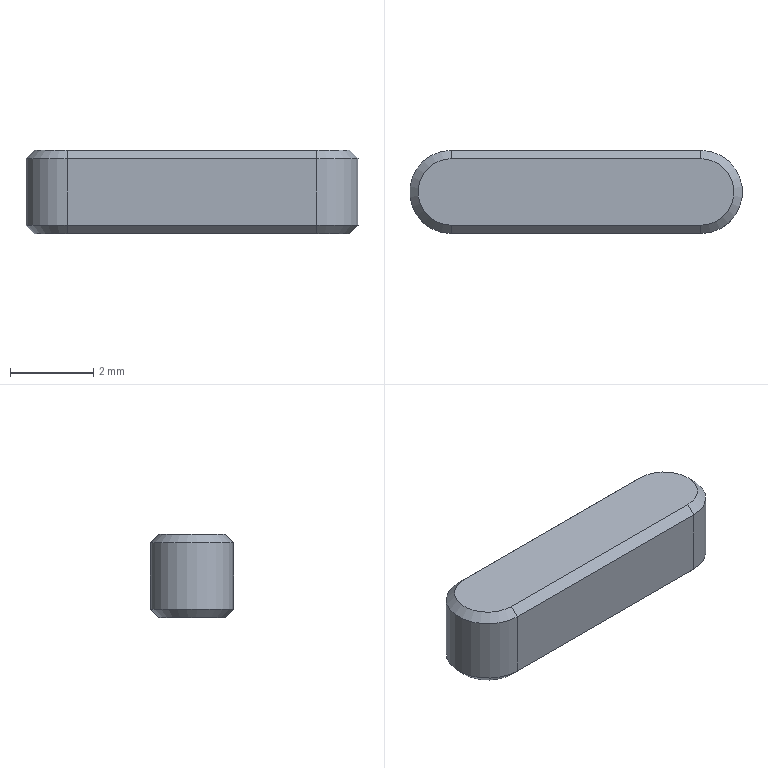Part | NX | features BREP 1, DATUM_CSYS 1 | 1 solid | 14 faces | box 8 x 2 x 2 mm | volume 29.569 mm3 | plane 8 | cone 4 | cylinder 2 | commonest cylinder face diameters 2 x2
STEP:
#1=CARTESIAN_POINT('',(3.,0.8,0.));
#2=VERTEX_POINT('',#1);
#3=CARTESIAN_POINT('',(-3.,0.8,0.));
#4=VERTEX_POINT('',#3);
#5=CARTESIAN_POINT('',(3.,0.8,0.));
#6=DIRECTION('',(-1.,0.,0.));
#7=VECTOR('',#6,1000.);
#8=LINE('',#5,#7);
#9=EDGE_CURVE('',#2,#4,#8,.T.);
#10=ORIENTED_EDGE('',*,*,#9,.F.);
#11=CARTESIAN_POINT('',(3.,-0.8,0.));
#12=VERTEX_POINT('',#11);
#13=CARTESIAN_POINT('',(3.,0.,0.));
#14=DIRECTION('',(0.,0.,1.));
#15=DIRECTION('',(0.,-1.,0.));
#16=AXIS2_PLACEMENT_3D('',#13,#14,#15);
#17=CIRCLE('',#16,0.8);
#18=EDGE_CURVE('',#12,#2,#17,.T.);
#19=ORIENTED_EDGE('',*,*,#18,.F.);
#20=CARTESIAN_POINT('',(-3.,-0.8,0.));
#21=VERTEX_POINT('',#20);
#22=CARTESIAN_POINT('',(-3.,-0.8,0.));
#23=DIRECTION('',(1.,0.,0.));
#24=VECTOR('',#23,1000.);
#25=LINE('',#22,#24);
#26=EDGE_CURVE('',#21,#12,#25,.T.);
#27=ORIENTED_EDGE('',*,*,#26,.F.);
#28=CARTESIAN_POINT('',(-3.,0.,0.));
#29=DIRECTION('',(0.,0.,1.));
#30=DIRECTION('',(0.,1.,0.));
#31=AXIS2_PLACEMENT_3D('',#28,#29,#30);
#32=CIRCLE('',#31,0.8);
#33=EDGE_CURVE('',#4,#21,#32,.T.);
#34=ORIENTED_EDGE('',*,*,#33,.F.);
#35=EDGE_LOOP('',(#10,#19,#27,#34));
#36=FACE_BOUND('',#35,.T.);
#37=CARTESIAN_POINT('',(0.,3.,0.));
#38=DIRECTION('',(0.,0.,1.));
#39=DIRECTION('',(-1.,0.,0.));
#40=AXIS2_PLACEMENT_3D('',#37,#38,#39);
#41=PLANE('',#40);
#42=ADVANCED_FACE('',(#36),#41,.F.);
#43=CARTESIAN_POINT('',(-3.,-0.8,2.));
#44=VERTEX_POINT('',#43);
#45=CARTESIAN_POINT('',(3.,-0.8,2.));
#46=VERTEX_POINT('',#45);
#47=CARTESIAN_POINT('',(-3.,-0.8,2.));
#48=DIRECTION('',(1.,0.,0.));
#49=VECTOR('',#48,1000.);
#50=LINE('',#47,#49);
#51=EDGE_CURVE('',#44,#46,#50,.T.);
#52=ORIENTED_EDGE('',*,*,#51,.T.);
#53=CARTESIAN_POINT('',(3.,0.8,2.));
#54=VERTEX_POINT('',#53);
#55=CARTESIAN_POINT('',(3.,0.,2.));
#56=DIRECTION('',(0.,0.,1.));
#57=DIRECTION('',(0.,-1.,0.));
#58=AXIS2_PLACEMENT_3D('',#55,#56,#57);
#59=CIRCLE('',#58,0.8);
#60=EDGE_CURVE('',#46,#54,#59,.T.);
#61=ORIENTED_EDGE('',*,*,#60,.T.);
#62=CARTESIAN_POINT('',(-3.,0.8,2.));
#63=VERTEX_POINT('',#62);
#64=CARTESIAN_POINT('',(3.,0.8,2.));
#65=DIRECTION('',(-1.,0.,0.));
#66=VECTOR('',#65,1000.);
#67=LINE('',#64,#66);
#68=EDGE_CURVE('',#54,#63,#67,.T.);
#69=ORIENTED_EDGE('',*,*,#68,.T.);
#70=CARTESIAN_POINT('',(-3.,0.,2.));
#71=DIRECTION('',(0.,0.,1.));
#72=DIRECTION('',(0.,1.,0.));
#73=AXIS2_PLACEMENT_3D('',#70,#71,#72);
#74=CIRCLE('',#73,0.8);
#75=EDGE_CURVE('',#63,#44,#74,.T.);
#76=ORIENTED_EDGE('',*,*,#75,.T.);
#77=EDGE_LOOP('',(#52,#61,#69,#76));
#78=FACE_BOUND('',#77,.T.);
#79=CARTESIAN_POINT('',(0.,3.,2.));
#80=DIRECTION('',(0.,0.,1.));
#81=DIRECTION('',(-1.,0.,0.));
#82=AXIS2_PLACEMENT_3D('',#79,#80,#81);
#83=PLANE('',#82);
#84=ADVANCED_FACE('',(#78),#83,.T.);
#85=CARTESIAN_POINT('',(-3.,-1.,0.2));
#86=VERTEX_POINT('',#85);
#87=CARTESIAN_POINT('',(-3.,-1.,1.8));
#88=VERTEX_POINT('',#87);
#89=CARTESIAN_POINT('',(-3.,-1.,0.2));
#90=DIRECTION('',(0.,0.,1.));
#91=VECTOR('',#90,1000.);
#92=LINE('',#89,#91);
#93=EDGE_CURVE('',#86,#88,#92,.T.);
#94=ORIENTED_EDGE('',*,*,#93,.F.);
#95=CARTESIAN_POINT('',(3.,-1.,0.2));
#96=VERTEX_POINT('',#95);
#97=CARTESIAN_POINT('',(-3.,-1.,0.2));
#98=DIRECTION('',(1.,0.,0.000000002));
#99=VECTOR('',#98,1000.);
#100=LINE('',#97,#99);
#101=EDGE_CURVE('',#86,#96,#100,.T.);
#102=ORIENTED_EDGE('',*,*,#101,.T.);
#103=CARTESIAN_POINT('',(3.,-1.,1.8));
#104=VERTEX_POINT('',#103);
#105=CARTESIAN_POINT('',(3.,-1.,0.2));
#106=DIRECTION('',(0.,0.,1.));
#107=VECTOR('',#106,1000.);
#108=LINE('',#105,#107);
#109=EDGE_CURVE('',#96,#104,#108,.T.);
#110=ORIENTED_EDGE('',*,*,#109,.T.);
#111=CARTESIAN_POINT('',(-3.,-1.,1.8));
#112=DIRECTION('',(1.,0.,0.));
#113=VECTOR('',#112,1000.);
#114=LINE('',#111,#113);
#115=EDGE_CURVE('',#88,#104,#114,.T.);
#116=ORIENTED_EDGE('',*,*,#115,.F.);
#117=EDGE_LOOP('',(#94,#102,#110,#116));
#118=FACE_BOUND('',#117,.T.);
#119=CARTESIAN_POINT('',(0.,-1.,1.));
#120=DIRECTION('',(0.,-1.,0.));
#121=DIRECTION('',(-1.,0.,0.));
#122=AXIS2_PLACEMENT_3D('',#119,#120,#121);
#123=PLANE('',#122);
#124=ADVANCED_FACE('',(#118),#123,.T.);
#125=CARTESIAN_POINT('',(3.,1.,0.2));
#126=VERTEX_POINT('',#125);
#127=CARTESIAN_POINT('',(3.,1.,1.8));
#128=VERTEX_POINT('',#127);
#129=CARTESIAN_POINT('',(3.,1.,0.2));
#130=DIRECTION('',(0.,0.,1.));
#131=VECTOR('',#130,1000.);
#132=LINE('',#129,#131);
#133=EDGE_CURVE('',#126,#128,#132,.T.);
#134=ORIENTED_EDGE('',*,*,#133,.T.);
#135=CARTESIAN_POINT('',(3.,0.,1.8));
#136=DIRECTION('',(0.000000014,0.,1.));
#137=DIRECTION('',(0.,-1.,0.));
#138=AXIS2_PLACEMENT_3D('',#135,#136,#137);
#139=CIRCLE('',#138,1.);
#140=EDGE_CURVE('',#104,#128,#139,.T.);
#141=ORIENTED_EDGE('',*,*,#140,.F.);
#142=ORIENTED_EDGE('',*,*,#109,.F.);
#143=CARTESIAN_POINT('',(3.,0.,0.2));
#144=DIRECTION('',(-0.000000019,0.,1.));
#145=DIRECTION('',(0.,-1.,0.));
#146=AXIS2_PLACEMENT_3D('',#143,#144,#145);
#147=CIRCLE('',#146,1.);
#148=EDGE_CURVE('',#96,#126,#147,.T.);
#149=ORIENTED_EDGE('',*,*,#148,.T.);
#150=EDGE_LOOP('',(#134,#141,#142,#149));
#151=FACE_BOUND('',#150,.T.);
#152=CARTESIAN_POINT('',(3.,0.,0.));
#153=DIRECTION('',(0.,0.,1.));
#154=DIRECTION('',(0.,1.,0.));
#155=AXIS2_PLACEMENT_3D('',#152,#153,#154);
#156=CYLINDRICAL_SURFACE('',#155,1.);
#157=ADVANCED_FACE('',(#151),#156,.T.);
#158=CARTESIAN_POINT('',(-3.,1.,0.2));
#159=VERTEX_POINT('',#158);
#160=CARTESIAN_POINT('',(-3.,1.,1.8));
#161=VERTEX_POINT('',#160);
#162=CARTESIAN_POINT('',(-3.,1.,0.2));
#163=DIRECTION('',(0.,0.,1.));
#164=VECTOR('',#163,1000.);
#165=LINE('',#162,#164);
#166=EDGE_CURVE('',#159,#161,#165,.T.);
#167=ORIENTED_EDGE('',*,*,#166,.T.);
#168=CARTESIAN_POINT('',(3.,1.,1.8));
#169=DIRECTION('',(-1.,0.,0.));
#170=VECTOR('',#169,1000.);
#171=LINE('',#168,#170);
#172=EDGE_CURVE('',#128,#161,#171,.T.);
#173=ORIENTED_EDGE('',*,*,#172,.F.);
#174=ORIENTED_EDGE('',*,*,#133,.F.);
#175=CARTESIAN_POINT('',(3.,1.,0.2));
#176=DIRECTION('',(-1.,0.,-0.000000002));
#177=VECTOR('',#176,1000.);
#178=LINE('',#175,#177);
#179=EDGE_CURVE('',#126,#159,#178,.T.);
#180=ORIENTED_EDGE('',*,*,#179,.T.);
#181=EDGE_LOOP('',(#167,#173,#174,#180));
#182=FACE_BOUND('',#181,.T.);
#183=CARTESIAN_POINT('',(0.,1.,1.));
#184=DIRECTION('',(0.,1.,0.));
#185=DIRECTION('',(1.,0.,0.));
#186=AXIS2_PLACEMENT_3D('',#183,#184,#185);
#187=PLANE('',#186);
#188=ADVANCED_FACE('',(#182),#187,.T.);
#189=ORIENTED_EDGE('',*,*,#166,.F.);
#190=CARTESIAN_POINT('',(-3.,0.,0.2));
#191=DIRECTION('',(0.000000014,0.,1.));
#192=DIRECTION('',(0.,1.,0.));
#193=AXIS2_PLACEMENT_3D('',#190,#191,#192);
#194=CIRCLE('',#193,1.);
#195=EDGE_CURVE('',#159,#86,#194,.T.);
#196=ORIENTED_EDGE('',*,*,#195,.T.);
#197=ORIENTED_EDGE('',*,*,#93,.T.);
#198=CARTESIAN_POINT('',(-3.,0.,1.8));
#199=DIRECTION('',(-0.000000013,0.,1.));
#200=DIRECTION('',(0.,1.,0.));
#201=AXIS2_PLACEMENT_3D('',#198,#199,#200);
#202=CIRCLE('',#201,1.);
#203=EDGE_CURVE('',#161,#88,#202,.T.);
#204=ORIENTED_EDGE('',*,*,#203,.F.);
#205=EDGE_LOOP('',(#189,#196,#197,#204));
#206=FACE_BOUND('',#205,.T.);
#207=CARTESIAN_POINT('',(-3.,0.,0.));
#208=DIRECTION('',(0.,0.,1.));
#209=DIRECTION('',(0.,-1.,0.));
#210=AXIS2_PLACEMENT_3D('',#207,#208,#209);
#211=CYLINDRICAL_SURFACE('',#210,1.);
#212=ADVANCED_FACE('',(#206),#211,.T.);
#213=ORIENTED_EDGE('',*,*,#195,.F.);
#214=CARTESIAN_POINT('',(-3.,0.8,0.));
#215=DIRECTION('',(0.,0.7071,0.7071));
#216=VECTOR('',#215,1000.);
#217=LINE('',#214,#216);
#218=EDGE_CURVE('',#4,#159,#217,.T.);
#219=ORIENTED_EDGE('',*,*,#218,.F.);
#220=ORIENTED_EDGE('',*,*,#33,.T.);
#221=CARTESIAN_POINT('',(-3.,-0.8,0.));
#222=DIRECTION('',(0.,-0.7071,0.7071));
#223=VECTOR('',#222,1000.);
#224=LINE('',#221,#223);
#225=EDGE_CURVE('',#21,#86,#224,.T.);
#226=ORIENTED_EDGE('',*,*,#225,.T.);
#227=EDGE_LOOP('',(#213,#219,#220,#226));
#228=FACE_BOUND('',#227,.T.);
#229=CARTESIAN_POINT('',(-3.,0.,0.));
#230=DIRECTION('',(0.,0.,1.));
#231=DIRECTION('',(0.,-1.,0.));
#232=AXIS2_PLACEMENT_3D('',#229,#230,#231);
#233=CONICAL_SURFACE('',#232,0.8,0.7854);
#234=ADVANCED_FACE('',(#228),#233,.T.);
#235=ORIENTED_EDGE('',*,*,#26,.T.);
#236=CARTESIAN_POINT('',(3.,-0.8,0.));
#237=DIRECTION('',(0.,-0.7071,0.7071));
#238=VECTOR('',#237,1000.);
#239=LINE('',#236,#238);
#240=EDGE_CURVE('',#12,#96,#239,.T.);
#241=ORIENTED_EDGE('',*,*,#240,.T.);
#242=ORIENTED_EDGE('',*,*,#101,.F.);
#243=ORIENTED_EDGE('',*,*,#225,.F.);
#244=EDGE_LOOP('',(#235,#241,#242,#243));
#245=FACE_BOUND('',#244,.T.);
#246=CARTESIAN_POINT('',(0.,-0.9,0.1));
#247=DIRECTION('',(0.,0.7071,0.7071));
#248=DIRECTION('',(0.,0.7071,-0.7071));
#249=AXIS2_PLACEMENT_3D('',#246,#247,#248);
#250=PLANE('',#249);
#251=ADVANCED_FACE('',(#245),#250,.F.);
#252=ORIENTED_EDGE('',*,*,#18,.T.);
#253=CARTESIAN_POINT('',(3.,0.8,0.));
#254=DIRECTION('',(0.,0.7071,0.7071));
#255=VECTOR('',#254,1000.);
#256=LINE('',#253,#255);
#257=EDGE_CURVE('',#2,#126,#256,.T.);
#258=ORIENTED_EDGE('',*,*,#257,.T.);
#259=ORIENTED_EDGE('',*,*,#148,.F.);
#260=ORIENTED_EDGE('',*,*,#240,.F.);
#261=EDGE_LOOP('',(#252,#258,#259,#260));
#262=FACE_BOUND('',#261,.T.);
#263=CARTESIAN_POINT('',(3.,0.,0.));
#264=DIRECTION('',(0.,0.,1.));
#265=DIRECTION('',(0.,1.,0.));
#266=AXIS2_PLACEMENT_3D('',#263,#264,#265);
#267=CONICAL_SURFACE('',#266,0.8,0.7854);
#268=ADVANCED_FACE('',(#262),#267,.T.);
#269=ORIENTED_EDGE('',*,*,#9,.T.);
#270=ORIENTED_EDGE('',*,*,#218,.T.);
#271=ORIENTED_EDGE('',*,*,#179,.F.);
#272=ORIENTED_EDGE('',*,*,#257,.F.);
#273=EDGE_LOOP('',(#269,#270,#271,#272));
#274=FACE_BOUND('',#273,.T.);
#275=CARTESIAN_POINT('',(0.,0.9,0.1));
#276=DIRECTION('',(0.,-0.7071,0.7071));
#277=DIRECTION('',(0.,-0.7071,-0.7071));
#278=AXIS2_PLACEMENT_3D('',#275,#276,#277);
#279=PLANE('',#278);
#280=ADVANCED_FACE('',(#274),#279,.F.);
#281=CARTESIAN_POINT('',(3.,-0.8,2.));
#282=DIRECTION('',(0.,-0.7071,-0.7071));
#283=VECTOR('',#282,1000.);
#284=LINE('',#281,#283);
#285=EDGE_CURVE('',#46,#104,#284,.T.);
#286=ORIENTED_EDGE('',*,*,#285,.F.);
#287=ORIENTED_EDGE('',*,*,#51,.F.);
#288=CARTESIAN_POINT('',(-3.,-0.8,2.));
#289=DIRECTION('',(0.,-0.7071,-0.7071));
#290=VECTOR('',#289,1000.);
#291=LINE('',#288,#290);
#292=EDGE_CURVE('',#44,#88,#291,.T.);
#293=ORIENTED_EDGE('',*,*,#292,.T.);
#294=ORIENTED_EDGE('',*,*,#115,.T.);
#295=EDGE_LOOP('',(#286,#287,#293,#294));
#296=FACE_BOUND('',#295,.T.);
#297=CARTESIAN_POINT('',(0.,-0.9,1.9));
#298=DIRECTION('',(0.,-0.7071,0.7071));
#299=DIRECTION('',(0.,0.7071,0.7071));
#300=AXIS2_PLACEMENT_3D('',#297,#298,#299);
#301=PLANE('',#300);
#302=ADVANCED_FACE('',(#296),#301,.T.);
#303=ORIENTED_EDGE('',*,*,#285,.T.);
#304=ORIENTED_EDGE('',*,*,#140,.T.);
#305=CARTESIAN_POINT('',(3.,0.8,2.));
#306=DIRECTION('',(0.,0.7071,-0.7071));
#307=VECTOR('',#306,1000.);
#308=LINE('',#305,#307);
#309=EDGE_CURVE('',#54,#128,#308,.T.);
#310=ORIENTED_EDGE('',*,*,#309,.F.);
#311=ORIENTED_EDGE('',*,*,#60,.F.);
#312=EDGE_LOOP('',(#303,#304,#310,#311));
#313=FACE_BOUND('',#312,.T.);
#314=CARTESIAN_POINT('',(3.,0.,2.));
#315=DIRECTION('',(0.,0.,-1.));
#316=DIRECTION('',(0.,1.,0.));
#317=AXIS2_PLACEMENT_3D('',#314,#315,#316);
#318=CONICAL_SURFACE('',#317,0.8,0.7854);
#319=ADVANCED_FACE('',(#313),#318,.T.);
#320=ORIENTED_EDGE('',*,*,#309,.T.);
#321=ORIENTED_EDGE('',*,*,#172,.T.);
#322=CARTESIAN_POINT('',(-3.,0.8,2.));
#323=DIRECTION('',(0.,0.7071,-0.7071));
#324=VECTOR('',#323,1000.);
#325=LINE('',#322,#324);
#326=EDGE_CURVE('',#63,#161,#325,.T.);
#327=ORIENTED_EDGE('',*,*,#326,.F.);
#328=ORIENTED_EDGE('',*,*,#68,.F.);
#329=EDGE_LOOP('',(#320,#321,#327,#328));
#330=FACE_BOUND('',#329,.T.);
#331=CARTESIAN_POINT('',(0.,0.9,1.9));
#332=DIRECTION('',(0.,0.7071,0.7071));
#333=DIRECTION('',(0.,-0.7071,0.7071));
#334=AXIS2_PLACEMENT_3D('',#331,#332,#333);
#335=PLANE('',#334);
#336=ADVANCED_FACE('',(#330),#335,.T.);
#337=ORIENTED_EDGE('',*,*,#326,.T.);
#338=ORIENTED_EDGE('',*,*,#203,.T.);
#339=ORIENTED_EDGE('',*,*,#292,.F.);
#340=ORIENTED_EDGE('',*,*,#75,.F.);
#341=EDGE_LOOP('',(#337,#338,#339,#340));
#342=FACE_BOUND('',#341,.T.);
#343=CARTESIAN_POINT('',(-3.,0.,2.));
#344=DIRECTION('',(0.,0.,-1.));
#345=DIRECTION('',(0.,-1.,0.));
#346=AXIS2_PLACEMENT_3D('',#343,#344,#345);
#347=CONICAL_SURFACE('',#346,0.8,0.7854);
#348=ADVANCED_FACE('',(#342),#347,.T.);
#349=CLOSED_SHELL('',(#42,#84,#124,#157,#188,#212,#234,#251,#268,#280,#302,#319,#336,#348));
#350=MANIFOLD_SOLID_BREP('',#349);
#351=(LENGTH_UNIT()NAMED_UNIT(*)SI_UNIT(.MILLI.,.METRE.));
#352=UNCERTAINTY_MEASURE_WITH_UNIT(LENGTH_MEASURE(0.00001),#351,'','');
#353=(NAMED_UNIT(*)PLANE_ANGLE_UNIT()SI_UNIT($,.RADIAN.));
#354=(NAMED_UNIT(*)SI_UNIT($,.STERADIAN.)SOLID_ANGLE_UNIT());
#355=(GEOMETRIC_REPRESENTATION_CONTEXT(3)GLOBAL_UNCERTAINTY_ASSIGNED_CONTEXT((#352))GLOBAL_UNIT_ASSIGNED_CONTEXT((#351,#353,#354))REPRESENTATION_CONTEXT('',''));
#356=ADVANCED_BREP_SHAPE_REPRESENTATION('',(#350),#355);